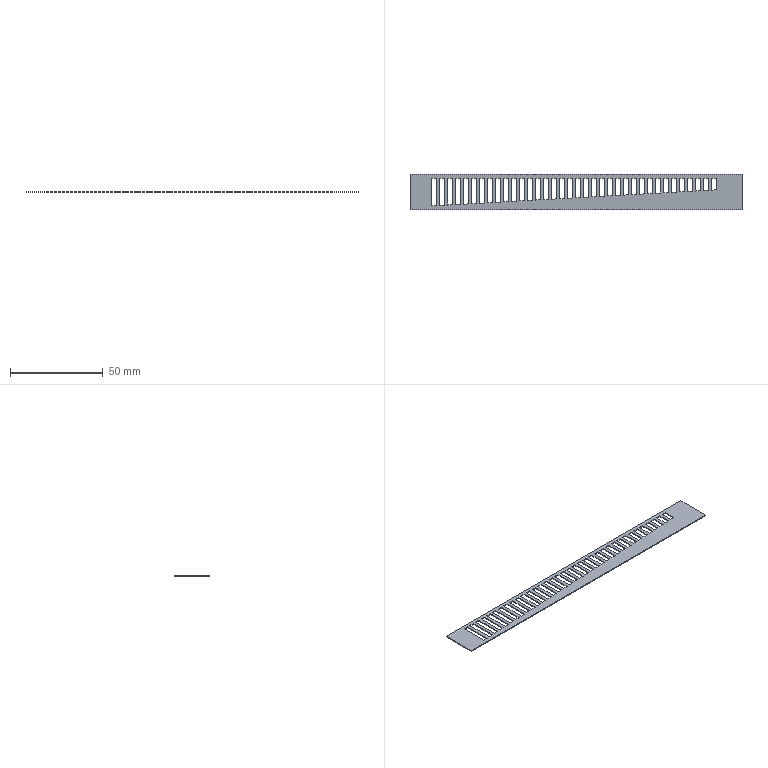Part | SolidWorks | features Extrusion 1, ICE 1 | 1 solid | 150 faces | box 178.5 x 19 x 0.5 mm | volume 1216 mm3 | plane 150